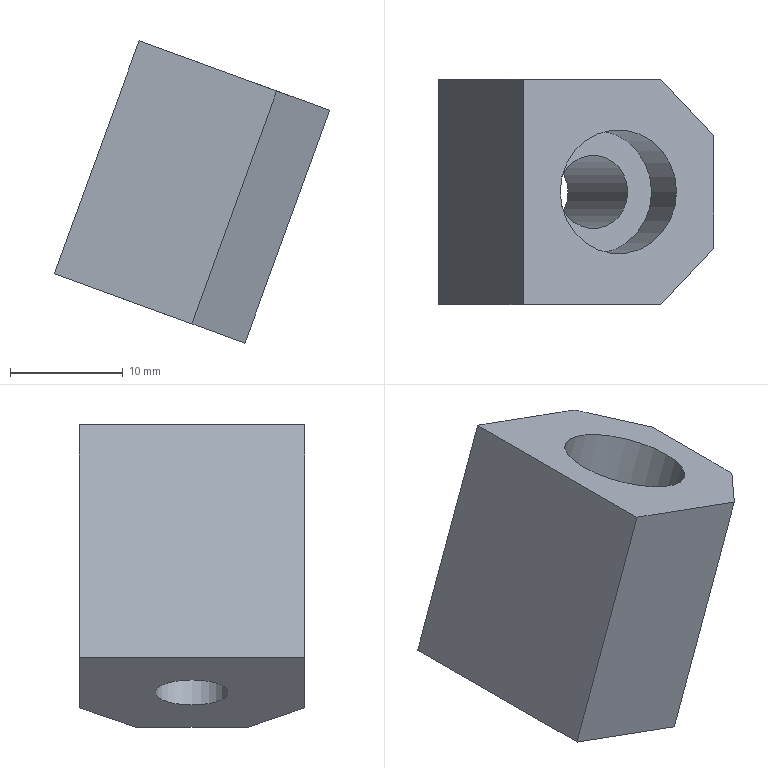Part | STEP file | P011002S002-010 | 1 solid | 11 faces | box 24.439 x 20 x 26.83 mm | volume 6238 mm3 | plane 9 | cylinder 2 | commonest cylinder face diameters 6.5 x1 11 x1
STEP:
#1=CARTESIAN_POINT('',(0.,0.,0.));
#2=DIRECTION('',(0.,0.,1.));
#3=DIRECTION('',(1.,0.,0.));
#4=AXIS2_PLACEMENT_3D('',#1,#2,#3);
#5=CARTESIAN_POINT('',(228.554,71.25,-64.902));
#6=VERTEX_POINT('',#5);
#7=CARTESIAN_POINT('',(240.77,71.25,-69.348));
#8=VERTEX_POINT('',#7);
#9=CARTESIAN_POINT('',(220.096,71.25,-61.824));
#10=DIRECTION('',(0.9397,0.,-0.342));
#11=VECTOR('',#10,1.);
#12=LINE('',#9,#11);
#13=CARTESIAN_POINT('',(220.096,-90.,-61.824));
#14=DIRECTION('',(0.342,0.,0.9397));
#15=DIRECTION('',(-0.9397,0.,0.342));
#16=AXIS2_PLACEMENT_3D('',#13,#14,#15);
#17=PLANE('',#16);
#18=CARTESIAN_POINT('',(0.,-161.25));
#19=DIRECTION('',(-1.,0.));
#20=VECTOR('',#19,1.);
#21=LINE('',#18,#20);
#22=(GEOMETRIC_REPRESENTATION_CONTEXT(2)PARAMETRIC_REPRESENTATION_CONTEXT()REPRESENTATION_CONTEXT('',''));
#23=DEFINITIONAL_REPRESENTATION('',(#21),#22);
#24=PCURVE('',#17,#23);
#25=CARTESIAN_POINT('',(229.238,71.25,-63.022));
#26=DIRECTION('',(0.,-1.,0.));
#27=DIRECTION('',(-0.9397,0.,0.342));
#28=AXIS2_PLACEMENT_3D('',#25,#26,#27);
#29=PLANE('',#28);
#30=CARTESIAN_POINT('',(9.,2.));
#31=DIRECTION('',(-1.,0.));
#32=VECTOR('',#31,1.);
#33=LINE('',#30,#32);
#34=(GEOMETRIC_REPRESENTATION_CONTEXT(2)PARAMETRIC_REPRESENTATION_CONTEXT()REPRESENTATION_CONTEXT('',''));
#35=DEFINITIONAL_REPRESENTATION('',(#33),#34);
#36=PCURVE('',#29,#35);
#37=SURFACE_CURVE('',#12,(#24,#36),.PCURVE_S1.);
#38=EDGE_CURVE('',#6,#8,#37,.T.);
#39=ORIENTED_EDGE('',*,*,#38,.F.);
#40=CARTESIAN_POINT('',(228.554,91.25,-64.902));
#41=VERTEX_POINT('',#40);
#42=CARTESIAN_POINT('',(228.554,-90.,-64.902));
#43=DIRECTION('',(0.,-1.,0.));
#44=VECTOR('',#43,1.);
#45=LINE('',#42,#44);
#46=CARTESIAN_POINT('',(-9.,0.));
#47=DIRECTION('',(0.,1.));
#48=VECTOR('',#47,1.);
#49=LINE('',#46,#48);
#50=(GEOMETRIC_REPRESENTATION_CONTEXT(2)PARAMETRIC_REPRESENTATION_CONTEXT()REPRESENTATION_CONTEXT('',''));
#51=DEFINITIONAL_REPRESENTATION('',(#49),#50);
#52=PCURVE('',#17,#51);
#53=CARTESIAN_POINT('',(229.238,86.25,-63.022));
#54=DIRECTION('',(-0.9397,0.,0.342));
#55=DIRECTION('',(-0.342,0.,-0.9397));
#56=AXIS2_PLACEMENT_3D('',#53,#54,#55);
#57=PLANE('',#56);
#58=CARTESIAN_POINT('',(2.,176.25));
#59=DIRECTION('',(0.,1.));
#60=VECTOR('',#59,1.);
#61=LINE('',#58,#60);
#62=(GEOMETRIC_REPRESENTATION_CONTEXT(2)PARAMETRIC_REPRESENTATION_CONTEXT()REPRESENTATION_CONTEXT('',''));
#63=DEFINITIONAL_REPRESENTATION('',(#61),#62);
#64=PCURVE('',#57,#63);
#65=SURFACE_CURVE('',#45,(#52,#64),.PCURVE_S1.);
#66=EDGE_CURVE('',#41,#6,#65,.T.);
#67=ORIENTED_EDGE('',*,*,#66,.F.);
#68=CARTESIAN_POINT('',(240.77,91.25,-69.348));
#69=VERTEX_POINT('',#68);
#70=CARTESIAN_POINT('',(228.554,91.25,-64.902));
#71=DIRECTION('',(0.9397,0.,-0.342));
#72=VECTOR('',#71,1.);
#73=LINE('',#70,#72);
#74=CARTESIAN_POINT('',(-9.,-181.25));
#75=DIRECTION('',(-1.,0.));
#76=VECTOR('',#75,1.);
#77=LINE('',#74,#76);
#78=(GEOMETRIC_REPRESENTATION_CONTEXT(2)PARAMETRIC_REPRESENTATION_CONTEXT()REPRESENTATION_CONTEXT('',''));
#79=DEFINITIONAL_REPRESENTATION('',(#77),#78);
#80=PCURVE('',#17,#79);
#81=CARTESIAN_POINT('',(229.238,91.25,-63.022));
#82=DIRECTION('',(0.,1.,0.));
#83=DIRECTION('',(0.9397,0.,-0.342));
#84=AXIS2_PLACEMENT_3D('',#81,#82,#83);
#85=PLANE('',#84);
#86=CARTESIAN_POINT('',(0.,2.));
#87=DIRECTION('',(1.,0.));
#88=VECTOR('',#87,1.);
#89=LINE('',#86,#88);
#90=(GEOMETRIC_REPRESENTATION_CONTEXT(2)PARAMETRIC_REPRESENTATION_CONTEXT()REPRESENTATION_CONTEXT('',''));
#91=DEFINITIONAL_REPRESENTATION('',(#89),#90);
#92=PCURVE('',#85,#91);
#93=SURFACE_CURVE('',#73,(#80,#92),.PCURVE_S1.);
#94=EDGE_CURVE('',#41,#69,#93,.T.);
#95=ORIENTED_EDGE('',*,*,#94,.T.);
#96=CARTESIAN_POINT('',(245.468,86.25,-71.058));
#97=VERTEX_POINT('',#96);
#98=CARTESIAN_POINT('',(315.593,11.625,-96.581));
#99=DIRECTION('',(-0.6645,0.7071,0.2418));
#100=VECTOR('',#99,1.);
#101=LINE('',#98,#100);
#102=CARTESIAN_POINT('',(-101.625,-101.625));
#103=DIRECTION('',(0.7071,-0.7071));
#104=VECTOR('',#103,1.);
#105=LINE('',#102,#104);
#106=(GEOMETRIC_REPRESENTATION_CONTEXT(2)PARAMETRIC_REPRESENTATION_CONTEXT()REPRESENTATION_CONTEXT('',''));
#107=DEFINITIONAL_REPRESENTATION('',(#105),#106);
#108=PCURVE('',#17,#107);
#109=CARTESIAN_POINT('',(241.454,91.25,-67.469));
#110=DIRECTION('',(-0.6645,-0.7071,0.2418));
#111=DIRECTION('',(-0.7287,0.6848,0.));
#112=AXIS2_PLACEMENT_3D('',#109,#110,#111);
#113=PLANE('',#112);
#114=CARTESIAN_POINT('',(-108.554,30.003));
#115=DIRECTION('',(0.9684,-0.2492));
#116=VECTOR('',#115,1.);
#117=LINE('',#114,#116);
#118=(GEOMETRIC_REPRESENTATION_CONTEXT(2)PARAMETRIC_REPRESENTATION_CONTEXT()REPRESENTATION_CONTEXT('',''));
#119=DEFINITIONAL_REPRESENTATION('',(#117),#118);
#120=PCURVE('',#113,#119);
#121=SURFACE_CURVE('',#101,(#108,#120),.PCURVE_S1.);
#122=EDGE_CURVE('',#97,#69,#121,.T.);
#123=ORIENTED_EDGE('',*,*,#122,.F.);
#124=CARTESIAN_POINT('',(245.468,76.25,-71.058));
#125=VERTEX_POINT('',#124);
#126=CARTESIAN_POINT('',(245.468,-90.,-71.058));
#127=DIRECTION('',(0.,1.,0.));
#128=VECTOR('',#127,1.);
#129=LINE('',#126,#128);
#130=CARTESIAN_POINT('',(-27.,0.));
#131=DIRECTION('',(0.,-1.));
#132=VECTOR('',#131,1.);
#133=LINE('',#130,#132);
#134=(GEOMETRIC_REPRESENTATION_CONTEXT(2)PARAMETRIC_REPRESENTATION_CONTEXT()REPRESENTATION_CONTEXT('',''));
#135=DEFINITIONAL_REPRESENTATION('',(#133),#134);
#136=PCURVE('',#17,#135);
#137=CARTESIAN_POINT('',(246.152,86.25,-69.179));
#138=DIRECTION('',(0.9397,0.,-0.342));
#139=DIRECTION('',(0.342,0.,0.9397));
#140=AXIS2_PLACEMENT_3D('',#137,#138,#139);
#141=PLANE('',#140);
#142=CARTESIAN_POINT('',(-2.,176.25));
#143=DIRECTION('',(0.,-1.));
#144=VECTOR('',#143,1.);
#145=LINE('',#142,#144);
#146=(GEOMETRIC_REPRESENTATION_CONTEXT(2)PARAMETRIC_REPRESENTATION_CONTEXT()REPRESENTATION_CONTEXT('',''));
#147=DEFINITIONAL_REPRESENTATION('',(#145),#146);
#148=PCURVE('',#141,#147);
#149=SURFACE_CURVE('',#129,(#136,#148),.PCURVE_S1.);
#150=EDGE_CURVE('',#125,#97,#149,.T.);
#151=ORIENTED_EDGE('',*,*,#150,.F.);
#152=CARTESIAN_POINT('',(154.67,-20.375,-38.01));
#153=DIRECTION('',(0.6645,0.7071,-0.2418));
#154=VECTOR('',#153,1.);
#155=LINE('',#152,#154);
#156=CARTESIAN_POINT('',(69.625,-69.625));
#157=DIRECTION('',(-0.7071,-0.7071));
#158=VECTOR('',#157,1.);
#159=LINE('',#156,#158);
#160=(GEOMETRIC_REPRESENTATION_CONTEXT(2)PARAMETRIC_REPRESENTATION_CONTEXT()REPRESENTATION_CONTEXT('',''));
#161=DEFINITIONAL_REPRESENTATION('',(#159),#160);
#162=PCURVE('',#17,#161);
#163=CARTESIAN_POINT('',(241.454,71.25,-67.469));
#164=DIRECTION('',(-0.6645,0.7071,0.2418));
#165=DIRECTION('',(0.7287,0.6848,0.));
#166=AXIS2_PLACEMENT_3D('',#163,#164,#165);
#167=PLANE('',#166);
#168=CARTESIAN_POINT('',(-125.986,-30.359));
#169=DIRECTION('',(0.9684,0.2492));
#170=VECTOR('',#169,1.);
#171=LINE('',#168,#170);
#172=(GEOMETRIC_REPRESENTATION_CONTEXT(2)PARAMETRIC_REPRESENTATION_CONTEXT()REPRESENTATION_CONTEXT('',''));
#173=DEFINITIONAL_REPRESENTATION('',(#171),#172);
#174=PCURVE('',#167,#173);
#175=SURFACE_CURVE('',#155,(#162,#174),.PCURVE_S1.);
#176=EDGE_CURVE('',#8,#125,#175,.T.);
#177=ORIENTED_EDGE('',*,*,#176,.F.);
#178=EDGE_LOOP('',(#39,#67,#95,#123,#151,#177));
#179=FACE_BOUND('',#178,.T.);
#180=CARTESIAN_POINT('',(233.957,81.25,-66.868));
#181=VERTEX_POINT('',#180);
#182=CARTESIAN_POINT('',(237.011,81.25,-67.98));
#183=DIRECTION('',(-0.342,0.,-0.9397));
#184=DIRECTION('',(-0.9397,0.,0.342));
#185=AXIS2_PLACEMENT_3D('',#182,#183,#184);
#186=CIRCLE('',#185,3.25);
#187=CARTESIAN_POINT('',(-14.75,-171.25));
#188=CARTESIAN_POINT('',(-14.75,-176.879));
#189=CARTESIAN_POINT('',(-19.625,-174.065));
#190=CARTESIAN_POINT('',(-24.5,-171.25));
#191=CARTESIAN_POINT('',(-19.625,-168.435));
#192=CARTESIAN_POINT('',(-14.75,-165.621));
#193=CARTESIAN_POINT('',(-14.75,-171.25));
#194=(BOUNDED_CURVE()B_SPLINE_CURVE(2,(#187,#188,#189,#190,#191,#192,#193),.UNSPECIFIED.,.T.,.F.)B_SPLINE_CURVE_WITH_KNOTS((1,2,2,2,2,1),(-2.094,0.,2.094,4.189,6.283,8.378),.UNSPECIFIED.)CURVE()GEOMETRIC_REPRESENTATION_ITEM()RATIONAL_B_SPLINE_CURVE((1.,0.5,1.,0.5,1.,0.5,1.))REPRESENTATION_ITEM(''));
#195=(GEOMETRIC_REPRESENTATION_CONTEXT(2)PARAMETRIC_REPRESENTATION_CONTEXT()REPRESENTATION_CONTEXT('',''));
#196=DEFINITIONAL_REPRESENTATION('',(#194),#195);
#197=PCURVE('',#17,#196);
#198=CARTESIAN_POINT('',(244.535,81.25,-47.307));
#199=DIRECTION('',(-0.342,0.,-0.9397));
#200=DIRECTION('',(0.9397,0.,-0.342));
#201=AXIS2_PLACEMENT_3D('',#198,#199,#200);
#202=CYLINDRICAL_SURFACE('',#201,3.25);
#203=CARTESIAN_POINT('',(3.142,22.));
#204=DIRECTION('',(1.,0.));
#205=VECTOR('',#204,1.);
#206=LINE('',#203,#205);
#207=(GEOMETRIC_REPRESENTATION_CONTEXT(2)PARAMETRIC_REPRESENTATION_CONTEXT()REPRESENTATION_CONTEXT('',''));
#208=DEFINITIONAL_REPRESENTATION('',(#206),#207);
#209=PCURVE('',#202,#208);
#210=SURFACE_CURVE('',#186,(#197,#209),.PCURVE_S1.);
#211=EDGE_CURVE('',#181,#181,#210,.T.);
#212=ORIENTED_EDGE('',*,*,#211,.F.);
#213=EDGE_LOOP('',(#212));
#214=FACE_BOUND('',#213,.T.);
#215=ADVANCED_FACE('',(#179,#214),#17,.F.);
#216=ORIENTED_EDGE('',*,*,#150,.T.);
#217=CARTESIAN_POINT('',(252.993,86.25,-50.385));
#218=VERTEX_POINT('',#217);
#219=CARTESIAN_POINT('',(246.152,86.25,-69.179));
#220=DIRECTION('',(-0.342,0.,-0.9397));
#221=VECTOR('',#220,1.);
#222=LINE('',#219,#221);
#223=CARTESIAN_POINT('',(0.,0.));
#224=DIRECTION('',(-1.,0.));
#225=VECTOR('',#224,1.);
#226=LINE('',#223,#225);
#227=(GEOMETRIC_REPRESENTATION_CONTEXT(2)PARAMETRIC_REPRESENTATION_CONTEXT()REPRESENTATION_CONTEXT('',''));
#228=DEFINITIONAL_REPRESENTATION('',(#226),#227);
#229=PCURVE('',#141,#228);
#230=CARTESIAN_POINT('',(-6.848,1.762));
#231=DIRECTION('',(0.2492,0.9684));
#232=VECTOR('',#231,1.);
#233=LINE('',#230,#232);
#234=(GEOMETRIC_REPRESENTATION_CONTEXT(2)PARAMETRIC_REPRESENTATION_CONTEXT()REPRESENTATION_CONTEXT('',''));
#235=DEFINITIONAL_REPRESENTATION('',(#233),#234);
#236=PCURVE('',#113,#235);
#237=SURFACE_CURVE('',#222,(#229,#236),.PCURVE_S1.);
#238=EDGE_CURVE('',#218,#97,#237,.T.);
#239=ORIENTED_EDGE('',*,*,#238,.F.);
#240=CARTESIAN_POINT('',(252.993,76.25,-50.385));
#241=VERTEX_POINT('',#240);
#242=CARTESIAN_POINT('',(252.993,86.25,-50.385));
#243=DIRECTION('',(0.,-1.,0.));
#244=VECTOR('',#243,1.);
#245=LINE('',#242,#244);
#246=CARTESIAN_POINT('',(20.,0.));
#247=DIRECTION('',(0.,1.));
#248=VECTOR('',#247,1.);
#249=LINE('',#246,#248);
#250=(GEOMETRIC_REPRESENTATION_CONTEXT(2)PARAMETRIC_REPRESENTATION_CONTEXT()REPRESENTATION_CONTEXT('',''));
#251=DEFINITIONAL_REPRESENTATION('',(#249),#250);
#252=PCURVE('',#141,#251);
#253=CARTESIAN_POINT('',(236.078,86.25,-44.229));
#254=DIRECTION('',(0.342,0.,0.9397));
#255=DIRECTION('',(-0.9397,0.,0.342));
#256=AXIS2_PLACEMENT_3D('',#253,#254,#255);
#257=PLANE('',#256);
#258=CARTESIAN_POINT('',(-18.,0.));
#259=DIRECTION('',(0.,1.));
#260=VECTOR('',#259,1.);
#261=LINE('',#258,#260);
#262=(GEOMETRIC_REPRESENTATION_CONTEXT(2)PARAMETRIC_REPRESENTATION_CONTEXT()REPRESENTATION_CONTEXT('',''));
#263=DEFINITIONAL_REPRESENTATION('',(#261),#262);
#264=PCURVE('',#257,#263);
#265=SURFACE_CURVE('',#245,(#252,#264),.PCURVE_S1.);
#266=EDGE_CURVE('',#218,#241,#265,.T.);
#267=ORIENTED_EDGE('',*,*,#266,.T.);
#268=CARTESIAN_POINT('',(246.152,76.25,-69.179));
#269=DIRECTION('',(0.342,0.,0.9397));
#270=VECTOR('',#269,1.);
#271=LINE('',#268,#270);
#272=CARTESIAN_POINT('',(0.,10.));
#273=DIRECTION('',(1.,0.));
#274=VECTOR('',#273,1.);
#275=LINE('',#272,#274);
#276=(GEOMETRIC_REPRESENTATION_CONTEXT(2)PARAMETRIC_REPRESENTATION_CONTEXT()REPRESENTATION_CONTEXT('',''));
#277=DEFINITIONAL_REPRESENTATION('',(#275),#276);
#278=PCURVE('',#141,#277);
#279=CARTESIAN_POINT('',(6.848,1.762));
#280=DIRECTION('',(0.2492,-0.9684));
#281=VECTOR('',#280,1.);
#282=LINE('',#279,#281);
#283=(GEOMETRIC_REPRESENTATION_CONTEXT(2)PARAMETRIC_REPRESENTATION_CONTEXT()REPRESENTATION_CONTEXT('',''));
#284=DEFINITIONAL_REPRESENTATION('',(#282),#283);
#285=PCURVE('',#167,#284);
#286=SURFACE_CURVE('',#271,(#278,#285),.PCURVE_S1.);
#287=EDGE_CURVE('',#125,#241,#286,.T.);
#288=ORIENTED_EDGE('',*,*,#287,.F.);
#289=EDGE_LOOP('',(#216,#239,#267,#288));
#290=FACE_BOUND('',#289,.T.);
#291=ADVANCED_FACE('',(#290),#141,.T.);
#292=CARTESIAN_POINT('',(236.078,71.25,-44.229));
#293=VERTEX_POINT('',#292);
#294=CARTESIAN_POINT('',(248.294,71.25,-48.675));
#295=VERTEX_POINT('',#294);
#296=CARTESIAN_POINT('',(236.078,71.25,-44.229));
#297=DIRECTION('',(0.9397,0.,-0.342));
#298=VECTOR('',#297,1.);
#299=LINE('',#296,#298);
#300=CARTESIAN_POINT('',(0.,-20.));
#301=DIRECTION('',(-1.,0.));
#302=VECTOR('',#301,1.);
#303=LINE('',#300,#302);
#304=(GEOMETRIC_REPRESENTATION_CONTEXT(2)PARAMETRIC_REPRESENTATION_CONTEXT()REPRESENTATION_CONTEXT('',''));
#305=DEFINITIONAL_REPRESENTATION('',(#303),#304);
#306=PCURVE('',#29,#305);
#307=CARTESIAN_POINT('',(0.,15.));
#308=DIRECTION('',(-1.,0.));
#309=VECTOR('',#308,1.);
#310=LINE('',#307,#309);
#311=(GEOMETRIC_REPRESENTATION_CONTEXT(2)PARAMETRIC_REPRESENTATION_CONTEXT()REPRESENTATION_CONTEXT('',''));
#312=DEFINITIONAL_REPRESENTATION('',(#310),#311);
#313=PCURVE('',#257,#312);
#314=SURFACE_CURVE('',#299,(#306,#313),.PCURVE_S1.);
#315=EDGE_CURVE('',#293,#295,#314,.T.);
#316=ORIENTED_EDGE('',*,*,#315,.F.);
#317=CARTESIAN_POINT('',(229.238,71.25,-63.022));
#318=DIRECTION('',(0.342,0.,0.9397));
#319=VECTOR('',#318,1.);
#320=LINE('',#317,#319);
#321=CARTESIAN_POINT('',(0.,0.));
#322=DIRECTION('',(0.,-1.));
#323=VECTOR('',#322,1.);
#324=LINE('',#321,#323);
#325=(GEOMETRIC_REPRESENTATION_CONTEXT(2)PARAMETRIC_REPRESENTATION_CONTEXT()REPRESENTATION_CONTEXT('',''));
#326=DEFINITIONAL_REPRESENTATION('',(#324),#325);
#327=PCURVE('',#29,#326);
#328=CARTESIAN_POINT('',(0.,15.));
#329=DIRECTION('',(-1.,0.));
#330=VECTOR('',#329,1.);
#331=LINE('',#328,#330);
#332=(GEOMETRIC_REPRESENTATION_CONTEXT(2)PARAMETRIC_REPRESENTATION_CONTEXT()REPRESENTATION_CONTEXT('',''));
#333=DEFINITIONAL_REPRESENTATION('',(#331),#332);
#334=PCURVE('',#57,#333);
#335=SURFACE_CURVE('',#320,(#327,#334),.PCURVE_S1.);
#336=EDGE_CURVE('',#6,#293,#335,.T.);
#337=ORIENTED_EDGE('',*,*,#336,.F.);
#338=ORIENTED_EDGE('',*,*,#38,.T.);
#339=CARTESIAN_POINT('',(241.454,71.25,-67.469));
#340=DIRECTION('',(-0.342,0.,-0.9397));
#341=VECTOR('',#340,1.);
#342=LINE('',#339,#341);
#343=CARTESIAN_POINT('',(-13.,0.));
#344=DIRECTION('',(0.,1.));
#345=VECTOR('',#344,1.);
#346=LINE('',#343,#345);
#347=(GEOMETRIC_REPRESENTATION_CONTEXT(2)PARAMETRIC_REPRESENTATION_CONTEXT()REPRESENTATION_CONTEXT('',''));
#348=DEFINITIONAL_REPRESENTATION('',(#346),#347);
#349=PCURVE('',#29,#348);
#350=CARTESIAN_POINT('',(0.,0.));
#351=DIRECTION('',(-0.2492,0.9684));
#352=VECTOR('',#351,1.);
#353=LINE('',#350,#352);
#354=(GEOMETRIC_REPRESENTATION_CONTEXT(2)PARAMETRIC_REPRESENTATION_CONTEXT()REPRESENTATION_CONTEXT('',''));
#355=DEFINITIONAL_REPRESENTATION('',(#353),#354);
#356=PCURVE('',#167,#355);
#357=SURFACE_CURVE('',#342,(#349,#356),.PCURVE_S1.);
#358=EDGE_CURVE('',#295,#8,#357,.T.);
#359=ORIENTED_EDGE('',*,*,#358,.F.);
#360=EDGE_LOOP('',(#316,#337,#338,#359));
#361=FACE_BOUND('',#360,.T.);
#362=ADVANCED_FACE('',(#361),#29,.T.);
#363=ORIENTED_EDGE('',*,*,#94,.F.);
#364=CARTESIAN_POINT('',(236.078,91.25,-44.229));
#365=VERTEX_POINT('',#364);
#366=CARTESIAN_POINT('',(229.238,91.25,-63.022));
#367=DIRECTION('',(-0.342,0.,-0.9397));
#368=VECTOR('',#367,1.);
#369=LINE('',#366,#368);
#370=CARTESIAN_POINT('',(0.,0.));
#371=DIRECTION('',(0.,1.));
#372=VECTOR('',#371,1.);
#373=LINE('',#370,#372);
#374=(GEOMETRIC_REPRESENTATION_CONTEXT(2)PARAMETRIC_REPRESENTATION_CONTEXT()REPRESENTATION_CONTEXT('',''));
#375=DEFINITIONAL_REPRESENTATION('',(#373),#374);
#376=PCURVE('',#85,#375);
#377=CARTESIAN_POINT('',(0.,-5.));
#378=DIRECTION('',(1.,0.));
#379=VECTOR('',#378,1.);
#380=LINE('',#377,#379);
#381=(GEOMETRIC_REPRESENTATION_CONTEXT(2)PARAMETRIC_REPRESENTATION_CONTEXT()REPRESENTATION_CONTEXT('',''));
#382=DEFINITIONAL_REPRESENTATION('',(#380),#381);
#383=PCURVE('',#57,#382);
#384=SURFACE_CURVE('',#369,(#376,#383),.PCURVE_S1.);
#385=EDGE_CURVE('',#365,#41,#384,.T.);
#386=ORIENTED_EDGE('',*,*,#385,.F.);
#387=CARTESIAN_POINT('',(248.294,91.25,-48.675));
#388=VERTEX_POINT('',#387);
#389=CARTESIAN_POINT('',(236.078,91.25,-44.229));
#390=DIRECTION('',(0.9397,0.,-0.342));
#391=VECTOR('',#390,1.);
#392=LINE('',#389,#391);
#393=CARTESIAN_POINT('',(0.,-20.));
#394=DIRECTION('',(1.,0.));
#395=VECTOR('',#394,1.);
#396=LINE('',#393,#395);
#397=(GEOMETRIC_REPRESENTATION_CONTEXT(2)PARAMETRIC_REPRESENTATION_CONTEXT()REPRESENTATION_CONTEXT('',''));
#398=DEFINITIONAL_REPRESENTATION('',(#396),#397);
#399=PCURVE('',#85,#398);
#400=CARTESIAN_POINT('',(0.,-5.));
#401=DIRECTION('',(-1.,0.));
#402=VECTOR('',#401,1.);
#403=LINE('',#400,#402);
#404=(GEOMETRIC_REPRESENTATION_CONTEXT(2)PARAMETRIC_REPRESENTATION_CONTEXT()REPRESENTATION_CONTEXT('',''));
#405=DEFINITIONAL_REPRESENTATION('',(#403),#404);
#406=PCURVE('',#257,#405);
#407=SURFACE_CURVE('',#392,(#399,#406),.PCURVE_S1.);
#408=EDGE_CURVE('',#365,#388,#407,.T.);
#409=ORIENTED_EDGE('',*,*,#408,.T.);
#410=CARTESIAN_POINT('',(241.454,91.25,-67.469));
#411=DIRECTION('',(0.342,0.,0.9397));
#412=VECTOR('',#411,1.);
#413=LINE('',#410,#412);
#414=CARTESIAN_POINT('',(13.,0.));
#415=DIRECTION('',(0.,-1.));
#416=VECTOR('',#415,1.);
#417=LINE('',#414,#416);
#418=(GEOMETRIC_REPRESENTATION_CONTEXT(2)PARAMETRIC_REPRESENTATION_CONTEXT()REPRESENTATION_CONTEXT('',''));
#419=DEFINITIONAL_REPRESENTATION('',(#417),#418);
#420=PCURVE('',#85,#419);
#421=CARTESIAN_POINT('',(0.,0.));
#422=DIRECTION('',(-0.2492,-0.9684));
#423=VECTOR('',#422,1.);
#424=LINE('',#421,#423);
#425=(GEOMETRIC_REPRESENTATION_CONTEXT(2)PARAMETRIC_REPRESENTATION_CONTEXT()REPRESENTATION_CONTEXT('',''));
#426=DEFINITIONAL_REPRESENTATION('',(#424),#425);
#427=PCURVE('',#113,#426);
#428=SURFACE_CURVE('',#413,(#420,#427),.PCURVE_S1.);
#429=EDGE_CURVE('',#69,#388,#428,.T.);
#430=ORIENTED_EDGE('',*,*,#429,.F.);
#431=EDGE_LOOP('',(#363,#386,#409,#430));
#432=FACE_BOUND('',#431,.T.);
#433=ADVANCED_FACE('',(#432),#85,.T.);
#434=CARTESIAN_POINT('',(236.078,86.25,-44.229));
#435=DIRECTION('',(0.,1.,0.));
#436=VECTOR('',#435,1.);
#437=LINE('',#434,#436);
#438=CARTESIAN_POINT('',(-20.,0.));
#439=DIRECTION('',(0.,-1.));
#440=VECTOR('',#439,1.);
#441=LINE('',#438,#440);
#442=(GEOMETRIC_REPRESENTATION_CONTEXT(2)PARAMETRIC_REPRESENTATION_CONTEXT()REPRESENTATION_CONTEXT('',''));
#443=DEFINITIONAL_REPRESENTATION('',(#441),#442);
#444=PCURVE('',#57,#443);
#445=CARTESIAN_POINT('',(0.,0.));
#446=DIRECTION('',(0.,-1.));
#447=VECTOR('',#446,1.);
#448=LINE('',#445,#447);
#449=(GEOMETRIC_REPRESENTATION_CONTEXT(2)PARAMETRIC_REPRESENTATION_CONTEXT()REPRESENTATION_CONTEXT('',''));
#450=DEFINITIONAL_REPRESENTATION('',(#448),#449);
#451=PCURVE('',#257,#450);
#452=SURFACE_CURVE('',#437,(#444,#451),.PCURVE_S1.);
#453=EDGE_CURVE('',#293,#365,#452,.T.);
#454=ORIENTED_EDGE('',*,*,#453,.T.);
#455=ORIENTED_EDGE('',*,*,#385,.T.);
#456=ORIENTED_EDGE('',*,*,#66,.T.);
#457=ORIENTED_EDGE('',*,*,#336,.T.);
#458=EDGE_LOOP('',(#454,#455,#456,#457));
#459=FACE_BOUND('',#458,.T.);
#460=ADVANCED_FACE('',(#459),#57,.T.);
#461=CARTESIAN_POINT('',(239.367,81.25,-45.426));
#462=VERTEX_POINT('',#461);
#463=CARTESIAN_POINT('',(244.535,81.25,-47.307));
#464=DIRECTION('',(-0.342,0.,-0.9397));
#465=DIRECTION('',(-0.9397,0.,0.342));
#466=AXIS2_PLACEMENT_3D('',#463,#464,#465);
#467=CIRCLE('',#466,5.5);
#468=CARTESIAN_POINT('',(-3.5,5.));
#469=CARTESIAN_POINT('',(-3.5,-4.526));
#470=CARTESIAN_POINT('',(-11.75,0.2369));
#471=CARTESIAN_POINT('',(-20.,5.));
#472=CARTESIAN_POINT('',(-11.75,9.763));
#473=CARTESIAN_POINT('',(-3.5,14.526));
#474=CARTESIAN_POINT('',(-3.5,5.));
#475=(BOUNDED_CURVE()B_SPLINE_CURVE(2,(#468,#469,#470,#471,#472,#473,#474),.UNSPECIFIED.,.T.,.F.)B_SPLINE_CURVE_WITH_KNOTS((1,2,2,2,2,1),(-2.094,0.,2.094,4.189,6.283,8.378),.UNSPECIFIED.)CURVE()GEOMETRIC_REPRESENTATION_ITEM()RATIONAL_B_SPLINE_CURVE((1.,0.5,1.,0.5,1.,0.5,1.))REPRESENTATION_ITEM(''));
#476=(GEOMETRIC_REPRESENTATION_CONTEXT(2)PARAMETRIC_REPRESENTATION_CONTEXT()REPRESENTATION_CONTEXT('',''));
#477=DEFINITIONAL_REPRESENTATION('',(#475),#476);
#478=PCURVE('',#257,#477);
#479=CARTESIAN_POINT('',(244.535,81.25,-47.307));
#480=DIRECTION('',(-0.342,0.,-0.9397));
#481=DIRECTION('',(0.9397,0.,-0.342));
#482=AXIS2_PLACEMENT_3D('',#479,#480,#481);
#483=CYLINDRICAL_SURFACE('',#482,5.5);
#484=CARTESIAN_POINT('',(3.142,0.));
#485=DIRECTION('',(1.,0.));
#486=VECTOR('',#485,1.);
#487=LINE('',#484,#486);
#488=(GEOMETRIC_REPRESENTATION_CONTEXT(2)PARAMETRIC_REPRESENTATION_CONTEXT()REPRESENTATION_CONTEXT('',''));
#489=DEFINITIONAL_REPRESENTATION('',(#487),#488);
#490=PCURVE('',#483,#489);
#491=SURFACE_CURVE('',#467,(#478,#490),.PCURVE_S1.);
#492=EDGE_CURVE('',#462,#462,#491,.T.);
#493=ORIENTED_EDGE('',*,*,#492,.T.);
#494=EDGE_LOOP('',(#493));
#495=FACE_BOUND('',#494,.T.);
#496=ORIENTED_EDGE('',*,*,#266,.F.);
#497=CARTESIAN_POINT('',(244.535,95.25,-47.307));
#498=DIRECTION('',(0.6645,-0.7071,-0.2418));
#499=VECTOR('',#498,1.);
#500=LINE('',#497,#499);
#501=CARTESIAN_POINT('',(-9.,-9.));
#502=DIRECTION('',(-0.7071,0.7071));
#503=VECTOR('',#502,1.);
#504=LINE('',#501,#503);
#505=(GEOMETRIC_REPRESENTATION_CONTEXT(2)PARAMETRIC_REPRESENTATION_CONTEXT()REPRESENTATION_CONTEXT('',''));
#506=DEFINITIONAL_REPRESENTATION('',(#504),#505);
#507=PCURVE('',#257,#506);
#508=CARTESIAN_POINT('',(0.4935,-20.779));
#509=DIRECTION('',(-0.9684,0.2492));
#510=VECTOR('',#509,1.);
#511=LINE('',#508,#510);
#512=(GEOMETRIC_REPRESENTATION_CONTEXT(2)PARAMETRIC_REPRESENTATION_CONTEXT()REPRESENTATION_CONTEXT('',''));
#513=DEFINITIONAL_REPRESENTATION('',(#511),#512);
#514=PCURVE('',#113,#513);
#515=SURFACE_CURVE('',#500,(#507,#514),.PCURVE_S1.);
#516=EDGE_CURVE('',#388,#218,#515,.T.);
#517=ORIENTED_EDGE('',*,*,#516,.F.);
#518=ORIENTED_EDGE('',*,*,#408,.F.);
#519=ORIENTED_EDGE('',*,*,#453,.F.);
#520=ORIENTED_EDGE('',*,*,#315,.T.);
#521=CARTESIAN_POINT('',(249.234,72.25,-49.017));
#522=DIRECTION('',(-0.6645,-0.7071,0.2418));
#523=VECTOR('',#522,1.);
#524=LINE('',#521,#523);
#525=CARTESIAN_POINT('',(-14.,14.));
#526=DIRECTION('',(0.7071,0.7071));
#527=VECTOR('',#526,1.);
#528=LINE('',#525,#527);
#529=(GEOMETRIC_REPRESENTATION_CONTEXT(2)PARAMETRIC_REPRESENTATION_CONTEXT()REPRESENTATION_CONTEXT('',''));
#530=DEFINITIONAL_REPRESENTATION('',(#528),#529);
#531=PCURVE('',#257,#530);
#532=CARTESIAN_POINT('',(6.354,-19.016));
#533=DIRECTION('',(-0.9684,-0.2492));
#534=VECTOR('',#533,1.);
#535=LINE('',#532,#534);
#536=(GEOMETRIC_REPRESENTATION_CONTEXT(2)PARAMETRIC_REPRESENTATION_CONTEXT()REPRESENTATION_CONTEXT('',''));
#537=DEFINITIONAL_REPRESENTATION('',(#535),#536);
#538=PCURVE('',#167,#537);
#539=SURFACE_CURVE('',#524,(#531,#538),.PCURVE_S1.);
#540=EDGE_CURVE('',#241,#295,#539,.T.);
#541=ORIENTED_EDGE('',*,*,#540,.F.);
#542=EDGE_LOOP('',(#496,#517,#518,#519,#520,#541));
#543=FACE_BOUND('',#542,.T.);
#544=ADVANCED_FACE('',(#495,#543),#257,.T.);
#545=ORIENTED_EDGE('',*,*,#540,.T.);
#546=ORIENTED_EDGE('',*,*,#358,.T.);
#547=ORIENTED_EDGE('',*,*,#176,.T.);
#548=ORIENTED_EDGE('',*,*,#287,.T.);
#549=EDGE_LOOP('',(#545,#546,#547,#548));
#550=FACE_BOUND('',#549,.T.);
#551=ADVANCED_FACE('',(#550),#167,.F.);
#552=ORIENTED_EDGE('',*,*,#122,.T.);
#553=ORIENTED_EDGE('',*,*,#429,.T.);
#554=ORIENTED_EDGE('',*,*,#516,.T.);
#555=ORIENTED_EDGE('',*,*,#238,.T.);
#556=EDGE_LOOP('',(#552,#553,#554,#555));
#557=FACE_BOUND('',#556,.T.);
#558=ADVANCED_FACE('',(#557),#113,.F.);
#559=ORIENTED_EDGE('',*,*,#211,.F.);
#560=CARTESIAN_POINT('',(239.258,81.25,-52.303));
#561=VERTEX_POINT('',#560);
#562=CARTESIAN_POINT('',(239.258,81.25,-52.303));
#563=CARTESIAN_POINT('',(233.957,81.25,-66.868));
#564=B_SPLINE_CURVE_WITH_KNOTS('',1,(#562,#563),.UNSPECIFIED.,.F.,.F.,(2,2),(6.5,22.),.PIECEWISE_BEZIER_KNOTS.);
#565=CARTESIAN_POINT('',(3.142,0.));
#566=DIRECTION('',(0.,1.));
#567=VECTOR('',#566,1.);
#568=LINE('',#565,#567);
#569=(GEOMETRIC_REPRESENTATION_CONTEXT(2)PARAMETRIC_REPRESENTATION_CONTEXT()REPRESENTATION_CONTEXT('',''));
#570=DEFINITIONAL_REPRESENTATION('',(#568),#569);
#571=PCURVE('',#202,#570);
#572=CARTESIAN_POINT('',(9.425,0.));
#573=DIRECTION('',(0.,1.));
#574=VECTOR('',#573,1.);
#575=LINE('',#572,#574);
#576=(GEOMETRIC_REPRESENTATION_CONTEXT(2)PARAMETRIC_REPRESENTATION_CONTEXT()REPRESENTATION_CONTEXT('',''));
#577=DEFINITIONAL_REPRESENTATION('',(#575),#576);
#578=PCURVE('',#202,#577);
#579=SEAM_CURVE('',#564,(#571,#578),.PCURVE_S1.);
#580=EDGE_CURVE('',#561,#181,#579,.T.);
#581=ORIENTED_EDGE('',*,*,#580,.F.);
#582=CARTESIAN_POINT('',(242.312,81.25,-53.415));
#583=DIRECTION('',(-0.342,0.,-0.9397));
#584=DIRECTION('',(-0.9397,0.,0.342));
#585=AXIS2_PLACEMENT_3D('',#582,#583,#584);
#586=CIRCLE('',#585,3.25);
#587=CARTESIAN_POINT('',(3.142,6.5));
#588=DIRECTION('',(1.,0.));
#589=VECTOR('',#588,1.);
#590=LINE('',#587,#589);
#591=(GEOMETRIC_REPRESENTATION_CONTEXT(2)PARAMETRIC_REPRESENTATION_CONTEXT()REPRESENTATION_CONTEXT('',''));
#592=DEFINITIONAL_REPRESENTATION('',(#590),#591);
#593=PCURVE('',#202,#592);
#594=CARTESIAN_POINT('',(242.312,81.25,-53.415));
#595=DIRECTION('',(0.342,0.,0.9397));
#596=DIRECTION('',(-0.9397,0.,0.342));
#597=AXIS2_PLACEMENT_3D('',#594,#595,#596);
#598=PLANE('',#597);
#599=CARTESIAN_POINT('',(3.25,0.));
#600=CARTESIAN_POINT('',(3.25,-5.629));
#601=CARTESIAN_POINT('',(-1.625,-2.815));
#602=CARTESIAN_POINT('',(-6.5,0.));
#603=CARTESIAN_POINT('',(-1.625,2.815));
#604=CARTESIAN_POINT('',(3.25,5.629));
#605=CARTESIAN_POINT('',(3.25,0.));
#606=(BOUNDED_CURVE()B_SPLINE_CURVE(2,(#599,#600,#601,#602,#603,#604,#605),.UNSPECIFIED.,.T.,.F.)B_SPLINE_CURVE_WITH_KNOTS((1,2,2,2,2,1),(-2.094,0.,2.094,4.189,6.283,8.378),.UNSPECIFIED.)CURVE()GEOMETRIC_REPRESENTATION_ITEM()RATIONAL_B_SPLINE_CURVE((1.,0.5,1.,0.5,1.,0.5,1.))REPRESENTATION_ITEM(''));
#607=(GEOMETRIC_REPRESENTATION_CONTEXT(2)PARAMETRIC_REPRESENTATION_CONTEXT()REPRESENTATION_CONTEXT('',''));
#608=DEFINITIONAL_REPRESENTATION('',(#606),#607);
#609=PCURVE('',#598,#608);
#610=SURFACE_CURVE('',#586,(#593,#609),.PCURVE_S1.);
#611=EDGE_CURVE('',#561,#561,#610,.T.);
#612=ORIENTED_EDGE('',*,*,#611,.T.);
#613=ORIENTED_EDGE('',*,*,#580,.T.);
#614=EDGE_LOOP('',(#559,#581,#612,#613));
#615=FACE_BOUND('',#614,.F.);
#616=ADVANCED_FACE('',(#615),#202,.F.);
#617=CARTESIAN_POINT('',(237.144,81.25,-51.534));
#618=VERTEX_POINT('',#617);
#619=CARTESIAN_POINT('',(242.312,81.25,-53.415));
#620=DIRECTION('',(-0.342,0.,-0.9397));
#621=DIRECTION('',(-0.9397,0.,0.342));
#622=AXIS2_PLACEMENT_3D('',#619,#620,#621);
#623=CIRCLE('',#622,5.5);
#624=CARTESIAN_POINT('',(5.5,0.));
#625=CARTESIAN_POINT('',(5.5,-9.526));
#626=CARTESIAN_POINT('',(-2.75,-4.763));
#627=CARTESIAN_POINT('',(-11.,0.));
#628=CARTESIAN_POINT('',(-2.75,4.763));
#629=CARTESIAN_POINT('',(5.5,9.526));
#630=CARTESIAN_POINT('',(5.5,0.));
#631=(BOUNDED_CURVE()B_SPLINE_CURVE(2,(#624,#625,#626,#627,#628,#629,#630),.UNSPECIFIED.,.T.,.F.)B_SPLINE_CURVE_WITH_KNOTS((1,2,2,2,2,1),(-2.094,0.,2.094,4.189,6.283,8.378),.UNSPECIFIED.)CURVE()GEOMETRIC_REPRESENTATION_ITEM()RATIONAL_B_SPLINE_CURVE((1.,0.5,1.,0.5,1.,0.5,1.))REPRESENTATION_ITEM(''));
#632=(GEOMETRIC_REPRESENTATION_CONTEXT(2)PARAMETRIC_REPRESENTATION_CONTEXT()REPRESENTATION_CONTEXT('',''));
#633=DEFINITIONAL_REPRESENTATION('',(#631),#632);
#634=PCURVE('',#598,#633);
#635=CARTESIAN_POINT('',(3.142,6.5));
#636=DIRECTION('',(1.,0.));
#637=VECTOR('',#636,1.);
#638=LINE('',#635,#637);
#639=(GEOMETRIC_REPRESENTATION_CONTEXT(2)PARAMETRIC_REPRESENTATION_CONTEXT()REPRESENTATION_CONTEXT('',''));
#640=DEFINITIONAL_REPRESENTATION('',(#638),#639);
#641=PCURVE('',#483,#640);
#642=SURFACE_CURVE('',#623,(#634,#641),.PCURVE_S1.);
#643=EDGE_CURVE('',#618,#618,#642,.T.);
#644=ORIENTED_EDGE('',*,*,#643,.F.);
#645=EDGE_LOOP('',(#644));
#646=FACE_BOUND('',#645,.T.);
#647=ORIENTED_EDGE('',*,*,#611,.T.);
#648=EDGE_LOOP('',(#647));
#649=FACE_BOUND('',#648,.T.);
#650=ADVANCED_FACE('',(#646,#649),#598,.T.);
#651=ORIENTED_EDGE('',*,*,#643,.F.);
#652=CARTESIAN_POINT('',(239.367,81.25,-45.426));
#653=CARTESIAN_POINT('',(237.144,81.25,-51.534));
#654=B_SPLINE_CURVE_WITH_KNOTS('',1,(#652,#653),.UNSPECIFIED.,.F.,.F.,(2,2),(0.,6.5),.PIECEWISE_BEZIER_KNOTS.);
#655=CARTESIAN_POINT('',(3.142,0.));
#656=DIRECTION('',(0.,1.));
#657=VECTOR('',#656,1.);
#658=LINE('',#655,#657);
#659=(GEOMETRIC_REPRESENTATION_CONTEXT(2)PARAMETRIC_REPRESENTATION_CONTEXT()REPRESENTATION_CONTEXT('',''));
#660=DEFINITIONAL_REPRESENTATION('',(#658),#659);
#661=PCURVE('',#483,#660);
#662=CARTESIAN_POINT('',(9.425,0.));
#663=DIRECTION('',(0.,1.));
#664=VECTOR('',#663,1.);
#665=LINE('',#662,#664);
#666=(GEOMETRIC_REPRESENTATION_CONTEXT(2)PARAMETRIC_REPRESENTATION_CONTEXT()REPRESENTATION_CONTEXT('',''));
#667=DEFINITIONAL_REPRESENTATION('',(#665),#666);
#668=PCURVE('',#483,#667);
#669=SEAM_CURVE('',#654,(#661,#668),.PCURVE_S1.);
#670=EDGE_CURVE('',#462,#618,#669,.T.);
#671=ORIENTED_EDGE('',*,*,#670,.F.);
#672=ORIENTED_EDGE('',*,*,#492,.T.);
#673=ORIENTED_EDGE('',*,*,#670,.T.);
#674=EDGE_LOOP('',(#651,#671,#672,#673));
#675=FACE_BOUND('',#674,.F.);
#676=ADVANCED_FACE('',(#675),#483,.F.);
#677=CLOSED_SHELL('',(#215,#291,#362,#433,#460,#544,#551,#558,#616,#650,#676));
#678=MANIFOLD_SOLID_BREP('',#677);
#679=(LENGTH_UNIT()NAMED_UNIT(*)SI_UNIT(.MILLI.,.METRE.));
#680=UNCERTAINTY_MEASURE_WITH_UNIT(LENGTH_MEASURE(0.000002),#679,'','');
#681=(NAMED_UNIT(*)PLANE_ANGLE_UNIT()SI_UNIT($,.RADIAN.));
#682=(NAMED_UNIT(*)SI_UNIT($,.STERADIAN.)SOLID_ANGLE_UNIT());
#683=(GEOMETRIC_REPRESENTATION_CONTEXT(3)GLOBAL_UNCERTAINTY_ASSIGNED_CONTEXT((#680))GLOBAL_UNIT_ASSIGNED_CONTEXT((#679,#681,#682))REPRESENTATION_CONTEXT('',''));
#684=ADVANCED_BREP_SHAPE_REPRESENTATION('',(#4,#678),#683);